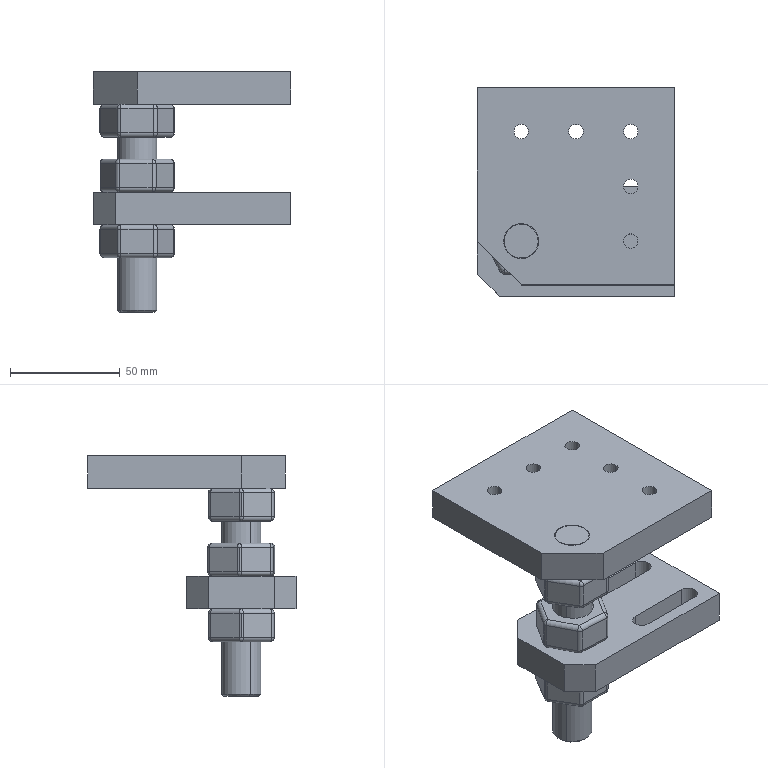Part | SolidWorks | 6 solids | 231 faces | box 90 x 95 x 110 mm | volume 212386 mm3 | cylinder 135 | plane 53 | sphere 36 | cone 4 | spline 3 | commonest cylinder face diameters 4 x57 18 x50 6.6 x10 12 x10 8.4 x4 15.5 x2